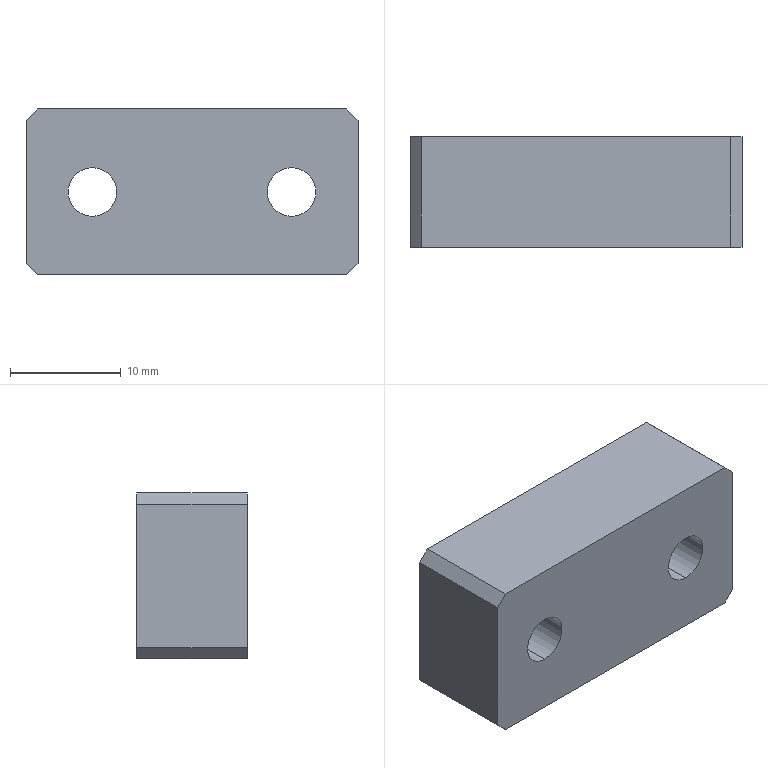Part | STEP file | PN_0004 | 1 solid | 14 faces | box 30 x 10 x 15 mm | volume 4176 mm3 | plane 10 | cylinder 4 | commonest cylinder face diameters 4.4 x4
STEP:
#1=CARTESIAN_POINT('',(0.,0.,0.));
#2=DIRECTION('',(0.,0.,1.));
#3=DIRECTION('',(1.,0.,0.));
#4=AXIS2_PLACEMENT_3D('',#1,#2,#3);
#5=CARTESIAN_POINT('',(9.,10.,-2.2));
#6=VERTEX_POINT('',#5);
#7=CARTESIAN_POINT('',(9.,0.,-2.2));
#8=VERTEX_POINT('',#7);
#9=CARTESIAN_POINT('',(9.,0.,-2.2));
#10=DIRECTION('',(0.,-1.,0.));
#11=VECTOR('',#10,1.);
#12=LINE('',#9,#11);
#13=CARTESIAN_POINT('',(9.,0.,0.));
#14=DIRECTION('',(0.,-1.,0.));
#15=DIRECTION('',(0.,0.,-1.));
#16=AXIS2_PLACEMENT_3D('',#13,#14,#15);
#17=CYLINDRICAL_SURFACE('',#16,2.2);
#18=CARTESIAN_POINT('',(6.283,0.));
#19=DIRECTION('',(0.,1.));
#20=VECTOR('',#19,1.);
#21=LINE('',#18,#20);
#22=(GEOMETRIC_REPRESENTATION_CONTEXT(2)PARAMETRIC_REPRESENTATION_CONTEXT()REPRESENTATION_CONTEXT('',''));
#23=DEFINITIONAL_REPRESENTATION('',(#21),#22);
#24=PCURVE('',#17,#23);
#25=CARTESIAN_POINT('',(9.,0.,0.));
#26=DIRECTION('',(0.,-1.,0.));
#27=DIRECTION('',(0.,0.,-1.));
#28=AXIS2_PLACEMENT_3D('',#25,#26,#27);
#29=CYLINDRICAL_SURFACE('',#28,2.2);
#30=CARTESIAN_POINT('',(0.,0.));
#31=DIRECTION('',(0.,1.));
#32=VECTOR('',#31,1.);
#33=LINE('',#30,#32);
#34=(GEOMETRIC_REPRESENTATION_CONTEXT(2)PARAMETRIC_REPRESENTATION_CONTEXT()REPRESENTATION_CONTEXT('',''));
#35=DEFINITIONAL_REPRESENTATION('',(#33),#34);
#36=PCURVE('',#29,#35);
#37=SURFACE_CURVE('',#12,(#24,#36),.PCURVE_S1.);
#38=EDGE_CURVE('',#6,#8,#37,.T.);
#39=ORIENTED_EDGE('',*,*,#38,.T.);
#40=CARTESIAN_POINT('',(9.,0.,2.2));
#41=VERTEX_POINT('',#40);
#42=CARTESIAN_POINT('',(9.,0.,0.));
#43=DIRECTION('',(0.,-1.,0.));
#44=DIRECTION('',(0.,0.,-1.));
#45=AXIS2_PLACEMENT_3D('',#42,#43,#44);
#46=CIRCLE('',#45,2.2);
#47=CARTESIAN_POINT('',(0.,0.));
#48=DIRECTION('',(1.,0.));
#49=VECTOR('',#48,1.);
#50=LINE('',#47,#49);
#51=(GEOMETRIC_REPRESENTATION_CONTEXT(2)PARAMETRIC_REPRESENTATION_CONTEXT()REPRESENTATION_CONTEXT('',''));
#52=DEFINITIONAL_REPRESENTATION('',(#50),#51);
#53=PCURVE('',#17,#52);
#54=CARTESIAN_POINT('',(0.,0.,0.));
#55=DIRECTION('',(0.,1.,0.));
#56=DIRECTION('',(0.,0.,1.));
#57=AXIS2_PLACEMENT_3D('',#54,#55,#56);
#58=PLANE('',#57);
#59=CARTESIAN_POINT('',(-2.2,9.));
#60=CARTESIAN_POINT('',(-2.2,12.811));
#61=CARTESIAN_POINT('',(1.1,10.905));
#62=CARTESIAN_POINT('',(4.4,9.));
#63=CARTESIAN_POINT('',(1.1,7.095));
#64=CARTESIAN_POINT('',(-2.2,5.189));
#65=CARTESIAN_POINT('',(-2.2,9.));
#66=(BOUNDED_CURVE()B_SPLINE_CURVE(2,(#59,#60,#61,#62,#63,#64,#65),.UNSPECIFIED.,.T.,.F.)B_SPLINE_CURVE_WITH_KNOTS((1,2,2,2,2,1),(-2.094,0.,2.094,4.189,6.283,8.378),.UNSPECIFIED.)CURVE()GEOMETRIC_REPRESENTATION_ITEM()RATIONAL_B_SPLINE_CURVE((1.,0.5,1.,0.5,1.,0.5,1.))REPRESENTATION_ITEM(''));
#67=(GEOMETRIC_REPRESENTATION_CONTEXT(2)PARAMETRIC_REPRESENTATION_CONTEXT()REPRESENTATION_CONTEXT('',''));
#68=DEFINITIONAL_REPRESENTATION('',(#66),#67);
#69=PCURVE('',#58,#68);
#70=SURFACE_CURVE('',#46,(#53,#69),.PCURVE_S1.);
#71=EDGE_CURVE('',#41,#8,#70,.T.);
#72=ORIENTED_EDGE('',*,*,#71,.F.);
#73=CARTESIAN_POINT('',(9.,10.,2.2));
#74=VERTEX_POINT('',#73);
#75=CARTESIAN_POINT('',(9.,0.,2.2));
#76=DIRECTION('',(0.,-1.,0.));
#77=VECTOR('',#76,1.);
#78=LINE('',#75,#77);
#79=CARTESIAN_POINT('',(3.142,0.));
#80=DIRECTION('',(0.,1.));
#81=VECTOR('',#80,1.);
#82=LINE('',#79,#81);
#83=(GEOMETRIC_REPRESENTATION_CONTEXT(2)PARAMETRIC_REPRESENTATION_CONTEXT()REPRESENTATION_CONTEXT('',''));
#84=DEFINITIONAL_REPRESENTATION('',(#82),#83);
#85=PCURVE('',#17,#84);
#86=CARTESIAN_POINT('',(3.142,0.));
#87=DIRECTION('',(0.,1.));
#88=VECTOR('',#87,1.);
#89=LINE('',#86,#88);
#90=(GEOMETRIC_REPRESENTATION_CONTEXT(2)PARAMETRIC_REPRESENTATION_CONTEXT()REPRESENTATION_CONTEXT('',''));
#91=DEFINITIONAL_REPRESENTATION('',(#89),#90);
#92=PCURVE('',#29,#91);
#93=SURFACE_CURVE('',#78,(#85,#92),.PCURVE_S1.);
#94=EDGE_CURVE('',#74,#41,#93,.T.);
#95=ORIENTED_EDGE('',*,*,#94,.F.);
#96=CARTESIAN_POINT('',(9.,10.,0.));
#97=DIRECTION('',(0.,-1.,0.));
#98=DIRECTION('',(0.,0.,-1.));
#99=AXIS2_PLACEMENT_3D('',#96,#97,#98);
#100=CIRCLE('',#99,2.2);
#101=CARTESIAN_POINT('',(0.,-10.));
#102=DIRECTION('',(1.,0.));
#103=VECTOR('',#102,1.);
#104=LINE('',#101,#103);
#105=(GEOMETRIC_REPRESENTATION_CONTEXT(2)PARAMETRIC_REPRESENTATION_CONTEXT()REPRESENTATION_CONTEXT('',''));
#106=DEFINITIONAL_REPRESENTATION('',(#104),#105);
#107=PCURVE('',#17,#106);
#108=CARTESIAN_POINT('',(0.,10.,0.));
#109=DIRECTION('',(0.,1.,0.));
#110=DIRECTION('',(0.,0.,1.));
#111=AXIS2_PLACEMENT_3D('',#108,#109,#110);
#112=PLANE('',#111);
#113=CARTESIAN_POINT('',(-2.2,9.));
#114=CARTESIAN_POINT('',(-2.2,12.811));
#115=CARTESIAN_POINT('',(1.1,10.905));
#116=CARTESIAN_POINT('',(4.4,9.));
#117=CARTESIAN_POINT('',(1.1,7.095));
#118=CARTESIAN_POINT('',(-2.2,5.189));
#119=CARTESIAN_POINT('',(-2.2,9.));
#120=(BOUNDED_CURVE()B_SPLINE_CURVE(2,(#113,#114,#115,#116,#117,#118,#119),.UNSPECIFIED.,.T.,.F.)B_SPLINE_CURVE_WITH_KNOTS((1,2,2,2,2,1),(-2.094,0.,2.094,4.189,6.283,8.378),.UNSPECIFIED.)CURVE()GEOMETRIC_REPRESENTATION_ITEM()RATIONAL_B_SPLINE_CURVE((1.,0.5,1.,0.5,1.,0.5,1.))REPRESENTATION_ITEM(''));
#121=(GEOMETRIC_REPRESENTATION_CONTEXT(2)PARAMETRIC_REPRESENTATION_CONTEXT()REPRESENTATION_CONTEXT('',''));
#122=DEFINITIONAL_REPRESENTATION('',(#120),#121);
#123=PCURVE('',#112,#122);
#124=SURFACE_CURVE('',#100,(#107,#123),.PCURVE_S1.);
#125=EDGE_CURVE('',#74,#6,#124,.T.);
#126=ORIENTED_EDGE('',*,*,#125,.T.);
#127=EDGE_LOOP('',(#39,#72,#95,#126));
#128=FACE_BOUND('',#127,.F.);
#129=ADVANCED_FACE('',(#128),#17,.F.);
#130=CARTESIAN_POINT('',(-9.,10.,-2.2));
#131=VERTEX_POINT('',#130);
#132=CARTESIAN_POINT('',(-9.,0.,-2.2));
#133=VERTEX_POINT('',#132);
#134=CARTESIAN_POINT('',(-9.,0.,-2.2));
#135=DIRECTION('',(0.,-1.,0.));
#136=VECTOR('',#135,1.);
#137=LINE('',#134,#136);
#138=CARTESIAN_POINT('',(-9.,0.,0.));
#139=DIRECTION('',(0.,-1.,0.));
#140=DIRECTION('',(0.,0.,-1.));
#141=AXIS2_PLACEMENT_3D('',#138,#139,#140);
#142=CYLINDRICAL_SURFACE('',#141,2.2);
#143=CARTESIAN_POINT('',(6.283,0.));
#144=DIRECTION('',(0.,1.));
#145=VECTOR('',#144,1.);
#146=LINE('',#143,#145);
#147=(GEOMETRIC_REPRESENTATION_CONTEXT(2)PARAMETRIC_REPRESENTATION_CONTEXT()REPRESENTATION_CONTEXT('',''));
#148=DEFINITIONAL_REPRESENTATION('',(#146),#147);
#149=PCURVE('',#142,#148);
#150=CARTESIAN_POINT('',(-9.,0.,0.));
#151=DIRECTION('',(0.,-1.,0.));
#152=DIRECTION('',(0.,0.,-1.));
#153=AXIS2_PLACEMENT_3D('',#150,#151,#152);
#154=CYLINDRICAL_SURFACE('',#153,2.2);
#155=CARTESIAN_POINT('',(0.,0.));
#156=DIRECTION('',(0.,1.));
#157=VECTOR('',#156,1.);
#158=LINE('',#155,#157);
#159=(GEOMETRIC_REPRESENTATION_CONTEXT(2)PARAMETRIC_REPRESENTATION_CONTEXT()REPRESENTATION_CONTEXT('',''));
#160=DEFINITIONAL_REPRESENTATION('',(#158),#159);
#161=PCURVE('',#154,#160);
#162=SURFACE_CURVE('',#137,(#149,#161),.PCURVE_S1.);
#163=EDGE_CURVE('',#131,#133,#162,.T.);
#164=ORIENTED_EDGE('',*,*,#163,.T.);
#165=CARTESIAN_POINT('',(-9.,0.,2.2));
#166=VERTEX_POINT('',#165);
#167=CARTESIAN_POINT('',(-9.,0.,0.));
#168=DIRECTION('',(0.,-1.,0.));
#169=DIRECTION('',(0.,0.,-1.));
#170=AXIS2_PLACEMENT_3D('',#167,#168,#169);
#171=CIRCLE('',#170,2.2);
#172=CARTESIAN_POINT('',(0.,0.));
#173=DIRECTION('',(1.,0.));
#174=VECTOR('',#173,1.);
#175=LINE('',#172,#174);
#176=(GEOMETRIC_REPRESENTATION_CONTEXT(2)PARAMETRIC_REPRESENTATION_CONTEXT()REPRESENTATION_CONTEXT('',''));
#177=DEFINITIONAL_REPRESENTATION('',(#175),#176);
#178=PCURVE('',#142,#177);
#179=CARTESIAN_POINT('',(-2.2,-9.));
#180=CARTESIAN_POINT('',(-2.2,-5.189));
#181=CARTESIAN_POINT('',(1.1,-7.095));
#182=CARTESIAN_POINT('',(4.4,-9.));
#183=CARTESIAN_POINT('',(1.1,-10.905));
#184=CARTESIAN_POINT('',(-2.2,-12.811));
#185=CARTESIAN_POINT('',(-2.2,-9.));
#186=(BOUNDED_CURVE()B_SPLINE_CURVE(2,(#179,#180,#181,#182,#183,#184,#185),.UNSPECIFIED.,.T.,.F.)B_SPLINE_CURVE_WITH_KNOTS((1,2,2,2,2,1),(-2.094,0.,2.094,4.189,6.283,8.378),.UNSPECIFIED.)CURVE()GEOMETRIC_REPRESENTATION_ITEM()RATIONAL_B_SPLINE_CURVE((1.,0.5,1.,0.5,1.,0.5,1.))REPRESENTATION_ITEM(''));
#187=(GEOMETRIC_REPRESENTATION_CONTEXT(2)PARAMETRIC_REPRESENTATION_CONTEXT()REPRESENTATION_CONTEXT('',''));
#188=DEFINITIONAL_REPRESENTATION('',(#186),#187);
#189=PCURVE('',#58,#188);
#190=SURFACE_CURVE('',#171,(#178,#189),.PCURVE_S1.);
#191=EDGE_CURVE('',#166,#133,#190,.T.);
#192=ORIENTED_EDGE('',*,*,#191,.F.);
#193=CARTESIAN_POINT('',(-9.,10.,2.2));
#194=VERTEX_POINT('',#193);
#195=CARTESIAN_POINT('',(-9.,0.,2.2));
#196=DIRECTION('',(0.,-1.,0.));
#197=VECTOR('',#196,1.);
#198=LINE('',#195,#197);
#199=CARTESIAN_POINT('',(3.142,0.));
#200=DIRECTION('',(0.,1.));
#201=VECTOR('',#200,1.);
#202=LINE('',#199,#201);
#203=(GEOMETRIC_REPRESENTATION_CONTEXT(2)PARAMETRIC_REPRESENTATION_CONTEXT()REPRESENTATION_CONTEXT('',''));
#204=DEFINITIONAL_REPRESENTATION('',(#202),#203);
#205=PCURVE('',#142,#204);
#206=CARTESIAN_POINT('',(3.142,0.));
#207=DIRECTION('',(0.,1.));
#208=VECTOR('',#207,1.);
#209=LINE('',#206,#208);
#210=(GEOMETRIC_REPRESENTATION_CONTEXT(2)PARAMETRIC_REPRESENTATION_CONTEXT()REPRESENTATION_CONTEXT('',''));
#211=DEFINITIONAL_REPRESENTATION('',(#209),#210);
#212=PCURVE('',#154,#211);
#213=SURFACE_CURVE('',#198,(#205,#212),.PCURVE_S1.);
#214=EDGE_CURVE('',#194,#166,#213,.T.);
#215=ORIENTED_EDGE('',*,*,#214,.F.);
#216=CARTESIAN_POINT('',(-9.,10.,0.));
#217=DIRECTION('',(0.,-1.,0.));
#218=DIRECTION('',(0.,0.,-1.));
#219=AXIS2_PLACEMENT_3D('',#216,#217,#218);
#220=CIRCLE('',#219,2.2);
#221=CARTESIAN_POINT('',(0.,-10.));
#222=DIRECTION('',(1.,0.));
#223=VECTOR('',#222,1.);
#224=LINE('',#221,#223);
#225=(GEOMETRIC_REPRESENTATION_CONTEXT(2)PARAMETRIC_REPRESENTATION_CONTEXT()REPRESENTATION_CONTEXT('',''));
#226=DEFINITIONAL_REPRESENTATION('',(#224),#225);
#227=PCURVE('',#142,#226);
#228=CARTESIAN_POINT('',(-2.2,-9.));
#229=CARTESIAN_POINT('',(-2.2,-5.189));
#230=CARTESIAN_POINT('',(1.1,-7.095));
#231=CARTESIAN_POINT('',(4.4,-9.));
#232=CARTESIAN_POINT('',(1.1,-10.905));
#233=CARTESIAN_POINT('',(-2.2,-12.811));
#234=CARTESIAN_POINT('',(-2.2,-9.));
#235=(BOUNDED_CURVE()B_SPLINE_CURVE(2,(#228,#229,#230,#231,#232,#233,#234),.UNSPECIFIED.,.T.,.F.)B_SPLINE_CURVE_WITH_KNOTS((1,2,2,2,2,1),(-2.094,0.,2.094,4.189,6.283,8.378),.UNSPECIFIED.)CURVE()GEOMETRIC_REPRESENTATION_ITEM()RATIONAL_B_SPLINE_CURVE((1.,0.5,1.,0.5,1.,0.5,1.))REPRESENTATION_ITEM(''));
#236=(GEOMETRIC_REPRESENTATION_CONTEXT(2)PARAMETRIC_REPRESENTATION_CONTEXT()REPRESENTATION_CONTEXT('',''));
#237=DEFINITIONAL_REPRESENTATION('',(#235),#236);
#238=PCURVE('',#112,#237);
#239=SURFACE_CURVE('',#220,(#227,#238),.PCURVE_S1.);
#240=EDGE_CURVE('',#194,#131,#239,.T.);
#241=ORIENTED_EDGE('',*,*,#240,.T.);
#242=EDGE_LOOP('',(#164,#192,#215,#241));
#243=FACE_BOUND('',#242,.F.);
#244=ADVANCED_FACE('',(#243),#142,.F.);
#245=CARTESIAN_POINT('',(15.,0.,6.5));
#246=VERTEX_POINT('',#245);
#247=CARTESIAN_POINT('',(15.,0.,-6.5));
#248=VERTEX_POINT('',#247);
#249=CARTESIAN_POINT('',(15.,0.,-7.5));
#250=DIRECTION('',(0.,0.,-1.));
#251=VECTOR('',#250,1.);
#252=LINE('',#249,#251);
#253=CARTESIAN_POINT('',(15.,10.,-7.5));
#254=DIRECTION('',(-1.,0.,0.));
#255=DIRECTION('',(0.,0.,1.));
#256=AXIS2_PLACEMENT_3D('',#253,#254,#255);
#257=PLANE('',#256);
#258=CARTESIAN_POINT('',(0.,-10.));
#259=DIRECTION('',(-1.,0.));
#260=VECTOR('',#259,1.);
#261=LINE('',#258,#260);
#262=(GEOMETRIC_REPRESENTATION_CONTEXT(2)PARAMETRIC_REPRESENTATION_CONTEXT()REPRESENTATION_CONTEXT('',''));
#263=DEFINITIONAL_REPRESENTATION('',(#261),#262);
#264=PCURVE('',#257,#263);
#265=CARTESIAN_POINT('',(-7.5,15.));
#266=DIRECTION('',(-1.,0.));
#267=VECTOR('',#266,1.);
#268=LINE('',#265,#267);
#269=(GEOMETRIC_REPRESENTATION_CONTEXT(2)PARAMETRIC_REPRESENTATION_CONTEXT()REPRESENTATION_CONTEXT('',''));
#270=DEFINITIONAL_REPRESENTATION('',(#268),#269);
#271=PCURVE('',#58,#270);
#272=SURFACE_CURVE('',#252,(#264,#271),.PCURVE_S1.);
#273=EDGE_CURVE('',#246,#248,#272,.T.);
#274=ORIENTED_EDGE('',*,*,#273,.T.);
#275=CARTESIAN_POINT('',(15.,10.,-6.5));
#276=VERTEX_POINT('',#275);
#277=CARTESIAN_POINT('',(15.,10.,-6.5));
#278=DIRECTION('',(0.,1.,0.));
#279=VECTOR('',#278,1.);
#280=LINE('',#277,#279);
#281=CARTESIAN_POINT('',(1.,0.));
#282=DIRECTION('',(0.,1.));
#283=VECTOR('',#282,1.);
#284=LINE('',#281,#283);
#285=(GEOMETRIC_REPRESENTATION_CONTEXT(2)PARAMETRIC_REPRESENTATION_CONTEXT()REPRESENTATION_CONTEXT('',''));
#286=DEFINITIONAL_REPRESENTATION('',(#284),#285);
#287=PCURVE('',#257,#286);
#288=CARTESIAN_POINT('',(14.,10.,-7.5));
#289=DIRECTION('',(-0.7071,0.,0.7071));
#290=DIRECTION('',(0.,-1.,0.));
#291=AXIS2_PLACEMENT_3D('',#288,#289,#290);
#292=PLANE('',#291);
#293=CARTESIAN_POINT('',(0.,1.414));
#294=DIRECTION('',(-1.,0.));
#295=VECTOR('',#294,1.);
#296=LINE('',#293,#295);
#297=(GEOMETRIC_REPRESENTATION_CONTEXT(2)PARAMETRIC_REPRESENTATION_CONTEXT()REPRESENTATION_CONTEXT('',''));
#298=DEFINITIONAL_REPRESENTATION('',(#296),#297);
#299=PCURVE('',#292,#298);
#300=SURFACE_CURVE('',#280,(#287,#299),.PCURVE_S1.);
#301=EDGE_CURVE('',#248,#276,#300,.T.);
#302=ORIENTED_EDGE('',*,*,#301,.T.);
#303=CARTESIAN_POINT('',(15.,10.,6.5));
#304=VERTEX_POINT('',#303);
#305=CARTESIAN_POINT('',(15.,10.,-7.5));
#306=DIRECTION('',(0.,0.,-1.));
#307=VECTOR('',#306,1.);
#308=LINE('',#305,#307);
#309=CARTESIAN_POINT('',(0.,0.));
#310=DIRECTION('',(-1.,0.));
#311=VECTOR('',#310,1.);
#312=LINE('',#309,#311);
#313=(GEOMETRIC_REPRESENTATION_CONTEXT(2)PARAMETRIC_REPRESENTATION_CONTEXT()REPRESENTATION_CONTEXT('',''));
#314=DEFINITIONAL_REPRESENTATION('',(#312),#313);
#315=PCURVE('',#257,#314);
#316=CARTESIAN_POINT('',(-7.5,15.));
#317=DIRECTION('',(-1.,0.));
#318=VECTOR('',#317,1.);
#319=LINE('',#316,#318);
#320=(GEOMETRIC_REPRESENTATION_CONTEXT(2)PARAMETRIC_REPRESENTATION_CONTEXT()REPRESENTATION_CONTEXT('',''));
#321=DEFINITIONAL_REPRESENTATION('',(#319),#320);
#322=PCURVE('',#112,#321);
#323=SURFACE_CURVE('',#308,(#315,#322),.PCURVE_S1.);
#324=EDGE_CURVE('',#304,#276,#323,.T.);
#325=ORIENTED_EDGE('',*,*,#324,.F.);
#326=CARTESIAN_POINT('',(15.,10.,6.5));
#327=DIRECTION('',(0.,-1.,0.));
#328=VECTOR('',#327,1.);
#329=LINE('',#326,#328);
#330=CARTESIAN_POINT('',(14.,0.));
#331=DIRECTION('',(0.,-1.));
#332=VECTOR('',#331,1.);
#333=LINE('',#330,#332);
#334=(GEOMETRIC_REPRESENTATION_CONTEXT(2)PARAMETRIC_REPRESENTATION_CONTEXT()REPRESENTATION_CONTEXT('',''));
#335=DEFINITIONAL_REPRESENTATION('',(#333),#334);
#336=PCURVE('',#257,#335);
#337=CARTESIAN_POINT('',(15.,10.,6.5));
#338=DIRECTION('',(-0.7071,0.,-0.7071));
#339=DIRECTION('',(0.,-1.,0.));
#340=AXIS2_PLACEMENT_3D('',#337,#338,#339);
#341=PLANE('',#340);
#342=CARTESIAN_POINT('',(0.,0.));
#343=DIRECTION('',(1.,0.));
#344=VECTOR('',#343,1.);
#345=LINE('',#342,#344);
#346=(GEOMETRIC_REPRESENTATION_CONTEXT(2)PARAMETRIC_REPRESENTATION_CONTEXT()REPRESENTATION_CONTEXT('',''));
#347=DEFINITIONAL_REPRESENTATION('',(#345),#346);
#348=PCURVE('',#341,#347);
#349=SURFACE_CURVE('',#329,(#336,#348),.PCURVE_S1.);
#350=EDGE_CURVE('',#304,#246,#349,.T.);
#351=ORIENTED_EDGE('',*,*,#350,.T.);
#352=EDGE_LOOP('',(#274,#302,#325,#351));
#353=FACE_BOUND('',#352,.T.);
#354=ADVANCED_FACE('',(#353),#257,.F.);
#355=CARTESIAN_POINT('',(14.,0.,-7.5));
#356=VERTEX_POINT('',#355);
#357=CARTESIAN_POINT('',(-14.,0.,-7.5));
#358=VERTEX_POINT('',#357);
#359=CARTESIAN_POINT('',(-15.,0.,-7.5));
#360=DIRECTION('',(-1.,0.,0.));
#361=VECTOR('',#360,1.);
#362=LINE('',#359,#361);
#363=CARTESIAN_POINT('',(-15.,10.,-7.5));
#364=DIRECTION('',(0.,0.,1.));
#365=DIRECTION('',(1.,0.,0.));
#366=AXIS2_PLACEMENT_3D('',#363,#364,#365);
#367=PLANE('',#366);
#368=CARTESIAN_POINT('',(0.,-10.));
#369=DIRECTION('',(-1.,0.));
#370=VECTOR('',#369,1.);
#371=LINE('',#368,#370);
#372=(GEOMETRIC_REPRESENTATION_CONTEXT(2)PARAMETRIC_REPRESENTATION_CONTEXT()REPRESENTATION_CONTEXT('',''));
#373=DEFINITIONAL_REPRESENTATION('',(#371),#372);
#374=PCURVE('',#367,#373);
#375=CARTESIAN_POINT('',(-7.5,-15.));
#376=DIRECTION('',(0.,-1.));
#377=VECTOR('',#376,1.);
#378=LINE('',#375,#377);
#379=(GEOMETRIC_REPRESENTATION_CONTEXT(2)PARAMETRIC_REPRESENTATION_CONTEXT()REPRESENTATION_CONTEXT('',''));
#380=DEFINITIONAL_REPRESENTATION('',(#378),#379);
#381=PCURVE('',#58,#380);
#382=SURFACE_CURVE('',#362,(#374,#381),.PCURVE_S1.);
#383=EDGE_CURVE('',#356,#358,#382,.T.);
#384=ORIENTED_EDGE('',*,*,#383,.T.);
#385=CARTESIAN_POINT('',(-14.,10.,-7.5));
#386=VERTEX_POINT('',#385);
#387=CARTESIAN_POINT('',(-14.,10.,-7.5));
#388=DIRECTION('',(0.,1.,0.));
#389=VECTOR('',#388,1.);
#390=LINE('',#387,#389);
#391=CARTESIAN_POINT('',(1.,0.));
#392=DIRECTION('',(0.,1.));
#393=VECTOR('',#392,1.);
#394=LINE('',#391,#393);
#395=(GEOMETRIC_REPRESENTATION_CONTEXT(2)PARAMETRIC_REPRESENTATION_CONTEXT()REPRESENTATION_CONTEXT('',''));
#396=DEFINITIONAL_REPRESENTATION('',(#394),#395);
#397=PCURVE('',#367,#396);
#398=CARTESIAN_POINT('',(-15.,10.,-6.5));
#399=DIRECTION('',(0.7071,0.,0.7071));
#400=DIRECTION('',(0.,-1.,0.));
#401=AXIS2_PLACEMENT_3D('',#398,#399,#400);
#402=PLANE('',#401);
#403=CARTESIAN_POINT('',(0.,1.414));
#404=DIRECTION('',(-1.,0.));
#405=VECTOR('',#404,1.);
#406=LINE('',#403,#405);
#407=(GEOMETRIC_REPRESENTATION_CONTEXT(2)PARAMETRIC_REPRESENTATION_CONTEXT()REPRESENTATION_CONTEXT('',''));
#408=DEFINITIONAL_REPRESENTATION('',(#406),#407);
#409=PCURVE('',#402,#408);
#410=SURFACE_CURVE('',#390,(#397,#409),.PCURVE_S1.);
#411=EDGE_CURVE('',#358,#386,#410,.T.);
#412=ORIENTED_EDGE('',*,*,#411,.T.);
#413=CARTESIAN_POINT('',(14.,10.,-7.5));
#414=VERTEX_POINT('',#413);
#415=CARTESIAN_POINT('',(-15.,10.,-7.5));
#416=DIRECTION('',(-1.,0.,0.));
#417=VECTOR('',#416,1.);
#418=LINE('',#415,#417);
#419=CARTESIAN_POINT('',(0.,0.));
#420=DIRECTION('',(-1.,0.));
#421=VECTOR('',#420,1.);
#422=LINE('',#419,#421);
#423=(GEOMETRIC_REPRESENTATION_CONTEXT(2)PARAMETRIC_REPRESENTATION_CONTEXT()REPRESENTATION_CONTEXT('',''));
#424=DEFINITIONAL_REPRESENTATION('',(#422),#423);
#425=PCURVE('',#367,#424);
#426=CARTESIAN_POINT('',(-7.5,-15.));
#427=DIRECTION('',(0.,-1.));
#428=VECTOR('',#427,1.);
#429=LINE('',#426,#428);
#430=(GEOMETRIC_REPRESENTATION_CONTEXT(2)PARAMETRIC_REPRESENTATION_CONTEXT()REPRESENTATION_CONTEXT('',''));
#431=DEFINITIONAL_REPRESENTATION('',(#429),#430);
#432=PCURVE('',#112,#431);
#433=SURFACE_CURVE('',#418,(#425,#432),.PCURVE_S1.);
#434=EDGE_CURVE('',#414,#386,#433,.T.);
#435=ORIENTED_EDGE('',*,*,#434,.F.);
#436=CARTESIAN_POINT('',(14.,10.,-7.5));
#437=DIRECTION('',(0.,-1.,0.));
#438=VECTOR('',#437,1.);
#439=LINE('',#436,#438);
#440=CARTESIAN_POINT('',(29.,0.));
#441=DIRECTION('',(0.,-1.));
#442=VECTOR('',#441,1.);
#443=LINE('',#440,#442);
#444=(GEOMETRIC_REPRESENTATION_CONTEXT(2)PARAMETRIC_REPRESENTATION_CONTEXT()REPRESENTATION_CONTEXT('',''));
#445=DEFINITIONAL_REPRESENTATION('',(#443),#444);
#446=PCURVE('',#367,#445);
#447=CARTESIAN_POINT('',(0.,0.));
#448=DIRECTION('',(1.,0.));
#449=VECTOR('',#448,1.);
#450=LINE('',#447,#449);
#451=(GEOMETRIC_REPRESENTATION_CONTEXT(2)PARAMETRIC_REPRESENTATION_CONTEXT()REPRESENTATION_CONTEXT('',''));
#452=DEFINITIONAL_REPRESENTATION('',(#450),#451);
#453=PCURVE('',#292,#452);
#454=SURFACE_CURVE('',#439,(#446,#453),.PCURVE_S1.);
#455=EDGE_CURVE('',#414,#356,#454,.T.);
#456=ORIENTED_EDGE('',*,*,#455,.T.);
#457=EDGE_LOOP('',(#384,#412,#435,#456));
#458=FACE_BOUND('',#457,.T.);
#459=ADVANCED_FACE('',(#458),#367,.F.);
#460=CARTESIAN_POINT('',(-15.,10.,-6.5));
#461=VERTEX_POINT('',#460);
#462=CARTESIAN_POINT('',(-15.,10.,6.5));
#463=VERTEX_POINT('',#462);
#464=CARTESIAN_POINT('',(-15.,10.,-7.5));
#465=DIRECTION('',(0.,0.,1.));
#466=VECTOR('',#465,1.);
#467=LINE('',#464,#466);
#468=CARTESIAN_POINT('',(-15.,10.,-7.5));
#469=DIRECTION('',(1.,0.,0.));
#470=DIRECTION('',(0.,0.,-1.));
#471=AXIS2_PLACEMENT_3D('',#468,#469,#470);
#472=PLANE('',#471);
#473=CARTESIAN_POINT('',(0.,0.));
#474=DIRECTION('',(-1.,0.));
#475=VECTOR('',#474,1.);
#476=LINE('',#473,#475);
#477=(GEOMETRIC_REPRESENTATION_CONTEXT(2)PARAMETRIC_REPRESENTATION_CONTEXT()REPRESENTATION_CONTEXT('',''));
#478=DEFINITIONAL_REPRESENTATION('',(#476),#477);
#479=PCURVE('',#472,#478);
#480=CARTESIAN_POINT('',(-7.5,-15.));
#481=DIRECTION('',(1.,0.));
#482=VECTOR('',#481,1.);
#483=LINE('',#480,#482);
#484=(GEOMETRIC_REPRESENTATION_CONTEXT(2)PARAMETRIC_REPRESENTATION_CONTEXT()REPRESENTATION_CONTEXT('',''));
#485=DEFINITIONAL_REPRESENTATION('',(#483),#484);
#486=PCURVE('',#112,#485);
#487=SURFACE_CURVE('',#467,(#479,#486),.PCURVE_S1.);
#488=EDGE_CURVE('',#461,#463,#487,.T.);
#489=ORIENTED_EDGE('',*,*,#488,.F.);
#490=CARTESIAN_POINT('',(-15.,0.,-6.5));
#491=VERTEX_POINT('',#490);
#492=CARTESIAN_POINT('',(-15.,10.,-6.5));
#493=DIRECTION('',(0.,-1.,0.));
#494=VECTOR('',#493,1.);
#495=LINE('',#492,#494);
#496=CARTESIAN_POINT('',(-1.,0.));
#497=DIRECTION('',(0.,-1.));
#498=VECTOR('',#497,1.);
#499=LINE('',#496,#498);
#500=(GEOMETRIC_REPRESENTATION_CONTEXT(2)PARAMETRIC_REPRESENTATION_CONTEXT()REPRESENTATION_CONTEXT('',''));
#501=DEFINITIONAL_REPRESENTATION('',(#499),#500);
#502=PCURVE('',#472,#501);
#503=CARTESIAN_POINT('',(0.,0.));
#504=DIRECTION('',(1.,0.));
#505=VECTOR('',#504,1.);
#506=LINE('',#503,#505);
#507=(GEOMETRIC_REPRESENTATION_CONTEXT(2)PARAMETRIC_REPRESENTATION_CONTEXT()REPRESENTATION_CONTEXT('',''));
#508=DEFINITIONAL_REPRESENTATION('',(#506),#507);
#509=PCURVE('',#402,#508);
#510=SURFACE_CURVE('',#495,(#502,#509),.PCURVE_S1.);
#511=EDGE_CURVE('',#461,#491,#510,.T.);
#512=ORIENTED_EDGE('',*,*,#511,.T.);
#513=CARTESIAN_POINT('',(-15.,0.,6.5));
#514=VERTEX_POINT('',#513);
#515=CARTESIAN_POINT('',(-15.,0.,-7.5));
#516=DIRECTION('',(0.,0.,1.));
#517=VECTOR('',#516,1.);
#518=LINE('',#515,#517);
#519=CARTESIAN_POINT('',(0.,-10.));
#520=DIRECTION('',(-1.,0.));
#521=VECTOR('',#520,1.);
#522=LINE('',#519,#521);
#523=(GEOMETRIC_REPRESENTATION_CONTEXT(2)PARAMETRIC_REPRESENTATION_CONTEXT()REPRESENTATION_CONTEXT('',''));
#524=DEFINITIONAL_REPRESENTATION('',(#522),#523);
#525=PCURVE('',#472,#524);
#526=CARTESIAN_POINT('',(-7.5,-15.));
#527=DIRECTION('',(1.,0.));
#528=VECTOR('',#527,1.);
#529=LINE('',#526,#528);
#530=(GEOMETRIC_REPRESENTATION_CONTEXT(2)PARAMETRIC_REPRESENTATION_CONTEXT()REPRESENTATION_CONTEXT('',''));
#531=DEFINITIONAL_REPRESENTATION('',(#529),#530);
#532=PCURVE('',#58,#531);
#533=SURFACE_CURVE('',#518,(#525,#532),.PCURVE_S1.);
#534=EDGE_CURVE('',#491,#514,#533,.T.);
#535=ORIENTED_EDGE('',*,*,#534,.T.);
#536=CARTESIAN_POINT('',(-15.,10.,6.5));
#537=DIRECTION('',(0.,1.,0.));
#538=VECTOR('',#537,1.);
#539=LINE('',#536,#538);
#540=CARTESIAN_POINT('',(-14.,0.));
#541=DIRECTION('',(0.,1.));
#542=VECTOR('',#541,1.);
#543=LINE('',#540,#542);
#544=(GEOMETRIC_REPRESENTATION_CONTEXT(2)PARAMETRIC_REPRESENTATION_CONTEXT()REPRESENTATION_CONTEXT('',''));
#545=DEFINITIONAL_REPRESENTATION('',(#543),#544);
#546=PCURVE('',#472,#545);
#547=CARTESIAN_POINT('',(-14.,10.,7.5));
#548=DIRECTION('',(0.7071,0.,-0.7071));
#549=DIRECTION('',(0.,-1.,0.));
#550=AXIS2_PLACEMENT_3D('',#547,#548,#549);
#551=PLANE('',#550);
#552=CARTESIAN_POINT('',(0.,1.414));
#553=DIRECTION('',(-1.,0.));
#554=VECTOR('',#553,1.);
#555=LINE('',#552,#554);
#556=(GEOMETRIC_REPRESENTATION_CONTEXT(2)PARAMETRIC_REPRESENTATION_CONTEXT()REPRESENTATION_CONTEXT('',''));
#557=DEFINITIONAL_REPRESENTATION('',(#555),#556);
#558=PCURVE('',#551,#557);
#559=SURFACE_CURVE('',#539,(#546,#558),.PCURVE_S1.);
#560=EDGE_CURVE('',#514,#463,#559,.T.);
#561=ORIENTED_EDGE('',*,*,#560,.T.);
#562=EDGE_LOOP('',(#489,#512,#535,#561));
#563=FACE_BOUND('',#562,.T.);
#564=ADVANCED_FACE('',(#563),#472,.F.);
#565=CARTESIAN_POINT('',(-14.,10.,7.5));
#566=VERTEX_POINT('',#565);
#567=CARTESIAN_POINT('',(14.,10.,7.5));
#568=VERTEX_POINT('',#567);
#569=CARTESIAN_POINT('',(-15.,10.,7.5));
#570=DIRECTION('',(1.,0.,0.));
#571=VECTOR('',#570,1.);
#572=LINE('',#569,#571);
#573=CARTESIAN_POINT('',(-15.,10.,7.5));
#574=DIRECTION('',(0.,0.,-1.));
#575=DIRECTION('',(-1.,0.,0.));
#576=AXIS2_PLACEMENT_3D('',#573,#574,#575);
#577=PLANE('',#576);
#578=CARTESIAN_POINT('',(0.,0.));
#579=DIRECTION('',(-1.,0.));
#580=VECTOR('',#579,1.);
#581=LINE('',#578,#580);
#582=(GEOMETRIC_REPRESENTATION_CONTEXT(2)PARAMETRIC_REPRESENTATION_CONTEXT()REPRESENTATION_CONTEXT('',''));
#583=DEFINITIONAL_REPRESENTATION('',(#581),#582);
#584=PCURVE('',#577,#583);
#585=CARTESIAN_POINT('',(7.5,-15.));
#586=DIRECTION('',(0.,1.));
#587=VECTOR('',#586,1.);
#588=LINE('',#585,#587);
#589=(GEOMETRIC_REPRESENTATION_CONTEXT(2)PARAMETRIC_REPRESENTATION_CONTEXT()REPRESENTATION_CONTEXT('',''));
#590=DEFINITIONAL_REPRESENTATION('',(#588),#589);
#591=PCURVE('',#112,#590);
#592=SURFACE_CURVE('',#572,(#584,#591),.PCURVE_S1.);
#593=EDGE_CURVE('',#566,#568,#592,.T.);
#594=ORIENTED_EDGE('',*,*,#593,.F.);
#595=CARTESIAN_POINT('',(-14.,0.,7.5));
#596=VERTEX_POINT('',#595);
#597=CARTESIAN_POINT('',(-14.,10.,7.5));
#598=DIRECTION('',(0.,-1.,0.));
#599=VECTOR('',#598,1.);
#600=LINE('',#597,#599);
#601=CARTESIAN_POINT('',(-1.,0.));
#602=DIRECTION('',(0.,-1.));
#603=VECTOR('',#602,1.);
#604=LINE('',#601,#603);
#605=(GEOMETRIC_REPRESENTATION_CONTEXT(2)PARAMETRIC_REPRESENTATION_CONTEXT()REPRESENTATION_CONTEXT('',''));
#606=DEFINITIONAL_REPRESENTATION('',(#604),#605);
#607=PCURVE('',#577,#606);
#608=CARTESIAN_POINT('',(0.,0.));
#609=DIRECTION('',(1.,0.));
#610=VECTOR('',#609,1.);
#611=LINE('',#608,#610);
#612=(GEOMETRIC_REPRESENTATION_CONTEXT(2)PARAMETRIC_REPRESENTATION_CONTEXT()REPRESENTATION_CONTEXT('',''));
#613=DEFINITIONAL_REPRESENTATION('',(#611),#612);
#614=PCURVE('',#551,#613);
#615=SURFACE_CURVE('',#600,(#607,#614),.PCURVE_S1.);
#616=EDGE_CURVE('',#566,#596,#615,.T.);
#617=ORIENTED_EDGE('',*,*,#616,.T.);
#618=CARTESIAN_POINT('',(14.,0.,7.5));
#619=VERTEX_POINT('',#618);
#620=CARTESIAN_POINT('',(-15.,0.,7.5));
#621=DIRECTION('',(1.,0.,0.));
#622=VECTOR('',#621,1.);
#623=LINE('',#620,#622);
#624=CARTESIAN_POINT('',(0.,-10.));
#625=DIRECTION('',(-1.,0.));
#626=VECTOR('',#625,1.);
#627=LINE('',#624,#626);
#628=(GEOMETRIC_REPRESENTATION_CONTEXT(2)PARAMETRIC_REPRESENTATION_CONTEXT()REPRESENTATION_CONTEXT('',''));
#629=DEFINITIONAL_REPRESENTATION('',(#627),#628);
#630=PCURVE('',#577,#629);
#631=CARTESIAN_POINT('',(7.5,-15.));
#632=DIRECTION('',(0.,1.));
#633=VECTOR('',#632,1.);
#634=LINE('',#631,#633);
#635=(GEOMETRIC_REPRESENTATION_CONTEXT(2)PARAMETRIC_REPRESENTATION_CONTEXT()REPRESENTATION_CONTEXT('',''));
#636=DEFINITIONAL_REPRESENTATION('',(#634),#635);
#637=PCURVE('',#58,#636);
#638=SURFACE_CURVE('',#623,(#630,#637),.PCURVE_S1.);
#639=EDGE_CURVE('',#596,#619,#638,.T.);
#640=ORIENTED_EDGE('',*,*,#639,.T.);
#641=CARTESIAN_POINT('',(14.,10.,7.5));
#642=DIRECTION('',(0.,1.,0.));
#643=VECTOR('',#642,1.);
#644=LINE('',#641,#643);
#645=CARTESIAN_POINT('',(-29.,0.));
#646=DIRECTION('',(0.,1.));
#647=VECTOR('',#646,1.);
#648=LINE('',#645,#647);
#649=(GEOMETRIC_REPRESENTATION_CONTEXT(2)PARAMETRIC_REPRESENTATION_CONTEXT()REPRESENTATION_CONTEXT('',''));
#650=DEFINITIONAL_REPRESENTATION('',(#648),#649);
#651=PCURVE('',#577,#650);
#652=CARTESIAN_POINT('',(0.,1.414));
#653=DIRECTION('',(-1.,0.));
#654=VECTOR('',#653,1.);
#655=LINE('',#652,#654);
#656=(GEOMETRIC_REPRESENTATION_CONTEXT(2)PARAMETRIC_REPRESENTATION_CONTEXT()REPRESENTATION_CONTEXT('',''));
#657=DEFINITIONAL_REPRESENTATION('',(#655),#656);
#658=PCURVE('',#341,#657);
#659=SURFACE_CURVE('',#644,(#651,#658),.PCURVE_S1.);
#660=EDGE_CURVE('',#619,#568,#659,.T.);
#661=ORIENTED_EDGE('',*,*,#660,.T.);
#662=EDGE_LOOP('',(#594,#617,#640,#661));
#663=FACE_BOUND('',#662,.T.);
#664=ADVANCED_FACE('',(#663),#577,.F.);
#665=CARTESIAN_POINT('',(9.,10.,0.));
#666=DIRECTION('',(0.,-1.,0.));
#667=DIRECTION('',(0.,0.,-1.));
#668=AXIS2_PLACEMENT_3D('',#665,#666,#667);
#669=CIRCLE('',#668,2.2);
#670=CARTESIAN_POINT('',(-2.2,9.));
#671=CARTESIAN_POINT('',(-2.2,12.811));
#672=CARTESIAN_POINT('',(1.1,10.905));
#673=CARTESIAN_POINT('',(4.4,9.));
#674=CARTESIAN_POINT('',(1.1,7.095));
#675=CARTESIAN_POINT('',(-2.2,5.189));
#676=CARTESIAN_POINT('',(-2.2,9.));
#677=(BOUNDED_CURVE()B_SPLINE_CURVE(2,(#670,#671,#672,#673,#674,#675,#676),.UNSPECIFIED.,.T.,.F.)B_SPLINE_CURVE_WITH_KNOTS((1,2,2,2,2,1),(-2.094,0.,2.094,4.189,6.283,8.378),.UNSPECIFIED.)CURVE()GEOMETRIC_REPRESENTATION_ITEM()RATIONAL_B_SPLINE_CURVE((1.,0.5,1.,0.5,1.,0.5,1.))REPRESENTATION_ITEM(''));
#678=(GEOMETRIC_REPRESENTATION_CONTEXT(2)PARAMETRIC_REPRESENTATION_CONTEXT()REPRESENTATION_CONTEXT('',''));
#679=DEFINITIONAL_REPRESENTATION('',(#677),#678);
#680=PCURVE('',#112,#679);
#681=CARTESIAN_POINT('',(0.,-10.));
#682=DIRECTION('',(1.,0.));
#683=VECTOR('',#682,1.);
#684=LINE('',#681,#683);
#685=(GEOMETRIC_REPRESENTATION_CONTEXT(2)PARAMETRIC_REPRESENTATION_CONTEXT()REPRESENTATION_CONTEXT('',''));
#686=DEFINITIONAL_REPRESENTATION('',(#684),#685);
#687=PCURVE('',#29,#686);
#688=SURFACE_CURVE('',#669,(#680,#687),.PCURVE_S1.);
#689=EDGE_CURVE('',#6,#74,#688,.T.);
#690=ORIENTED_EDGE('',*,*,#689,.T.);
#691=ORIENTED_EDGE('',*,*,#125,.T.);
#692=EDGE_LOOP('',(#690,#691));
#693=FACE_BOUND('',#692,.T.);
#694=CARTESIAN_POINT('',(-9.,10.,0.));
#695=DIRECTION('',(0.,-1.,0.));
#696=DIRECTION('',(0.,0.,-1.));
#697=AXIS2_PLACEMENT_3D('',#694,#695,#696);
#698=CIRCLE('',#697,2.2);
#699=CARTESIAN_POINT('',(-2.2,-9.));
#700=CARTESIAN_POINT('',(-2.2,-5.189));
#701=CARTESIAN_POINT('',(1.1,-7.095));
#702=CARTESIAN_POINT('',(4.4,-9.));
#703=CARTESIAN_POINT('',(1.1,-10.905));
#704=CARTESIAN_POINT('',(-2.2,-12.811));
#705=CARTESIAN_POINT('',(-2.2,-9.));
#706=(BOUNDED_CURVE()B_SPLINE_CURVE(2,(#699,#700,#701,#702,#703,#704,#705),.UNSPECIFIED.,.T.,.F.)B_SPLINE_CURVE_WITH_KNOTS((1,2,2,2,2,1),(-2.094,0.,2.094,4.189,6.283,8.378),.UNSPECIFIED.)CURVE()GEOMETRIC_REPRESENTATION_ITEM()RATIONAL_B_SPLINE_CURVE((1.,0.5,1.,0.5,1.,0.5,1.))REPRESENTATION_ITEM(''));
#707=(GEOMETRIC_REPRESENTATION_CONTEXT(2)PARAMETRIC_REPRESENTATION_CONTEXT()REPRESENTATION_CONTEXT('',''));
#708=DEFINITIONAL_REPRESENTATION('',(#706),#707);
#709=PCURVE('',#112,#708);
#710=CARTESIAN_POINT('',(0.,-10.));
#711=DIRECTION('',(1.,0.));
#712=VECTOR('',#711,1.);
#713=LINE('',#710,#712);
#714=(GEOMETRIC_REPRESENTATION_CONTEXT(2)PARAMETRIC_REPRESENTATION_CONTEXT()REPRESENTATION_CONTEXT('',''));
#715=DEFINITIONAL_REPRESENTATION('',(#713),#714);
#716=PCURVE('',#154,#715);
#717=SURFACE_CURVE('',#698,(#709,#716),.PCURVE_S1.);
#718=EDGE_CURVE('',#131,#194,#717,.T.);
#719=ORIENTED_EDGE('',*,*,#718,.T.);
#720=ORIENTED_EDGE('',*,*,#240,.T.);
#721=EDGE_LOOP('',(#719,#720));
#722=FACE_BOUND('',#721,.T.);
#723=ORIENTED_EDGE('',*,*,#434,.T.);
#724=CARTESIAN_POINT('',(-10.75,10.,-10.75));
#725=DIRECTION('',(-0.7071,0.,0.7071));
#726=VECTOR('',#725,1.);
#727=LINE('',#724,#726);
#728=CARTESIAN_POINT('',(-10.75,-10.75));
#729=DIRECTION('',(0.7071,-0.7071));
#730=VECTOR('',#729,1.);
#731=LINE('',#728,#730);
#732=(GEOMETRIC_REPRESENTATION_CONTEXT(2)PARAMETRIC_REPRESENTATION_CONTEXT()REPRESENTATION_CONTEXT('',''));
#733=DEFINITIONAL_REPRESENTATION('',(#731),#732);
#734=PCURVE('',#112,#733);
#735=CARTESIAN_POINT('',(0.,6.01));
#736=DIRECTION('',(0.,-1.));
#737=VECTOR('',#736,1.);
#738=LINE('',#735,#737);
#739=(GEOMETRIC_REPRESENTATION_CONTEXT(2)PARAMETRIC_REPRESENTATION_CONTEXT()REPRESENTATION_CONTEXT('',''));
#740=DEFINITIONAL_REPRESENTATION('',(#738),#739);
#741=PCURVE('',#402,#740);
#742=SURFACE_CURVE('',#727,(#734,#741),.PCURVE_S1.);
#743=EDGE_CURVE('',#386,#461,#742,.T.);
#744=ORIENTED_EDGE('',*,*,#743,.T.);
#745=ORIENTED_EDGE('',*,*,#488,.T.);
#746=CARTESIAN_POINT('',(-10.75,10.,10.75));
#747=DIRECTION('',(0.7071,0.,0.7071));
#748=VECTOR('',#747,1.);
#749=LINE('',#746,#748);
#750=CARTESIAN_POINT('',(10.75,-10.75));
#751=DIRECTION('',(0.7071,0.7071));
#752=VECTOR('',#751,1.);
#753=LINE('',#750,#752);
#754=(GEOMETRIC_REPRESENTATION_CONTEXT(2)PARAMETRIC_REPRESENTATION_CONTEXT()REPRESENTATION_CONTEXT('',''));
#755=DEFINITIONAL_REPRESENTATION('',(#753),#754);
#756=PCURVE('',#112,#755);
#757=CARTESIAN_POINT('',(0.,-4.596));
#758=DIRECTION('',(0.,-1.));
#759=VECTOR('',#758,1.);
#760=LINE('',#757,#759);
#761=(GEOMETRIC_REPRESENTATION_CONTEXT(2)PARAMETRIC_REPRESENTATION_CONTEXT()REPRESENTATION_CONTEXT('',''));
#762=DEFINITIONAL_REPRESENTATION('',(#760),#761);
#763=PCURVE('',#551,#762);
#764=SURFACE_CURVE('',#749,(#756,#763),.PCURVE_S1.);
#765=EDGE_CURVE('',#463,#566,#764,.T.);
#766=ORIENTED_EDGE('',*,*,#765,.T.);
#767=ORIENTED_EDGE('',*,*,#593,.T.);
#768=CARTESIAN_POINT('',(10.75,10.,10.75));
#769=DIRECTION('',(0.7071,0.,-0.7071));
#770=VECTOR('',#769,1.);
#771=LINE('',#768,#770);
#772=CARTESIAN_POINT('',(10.75,10.75));
#773=DIRECTION('',(-0.7071,0.7071));
#774=VECTOR('',#773,1.);
#775=LINE('',#772,#774);
#776=(GEOMETRIC_REPRESENTATION_CONTEXT(2)PARAMETRIC_REPRESENTATION_CONTEXT()REPRESENTATION_CONTEXT('',''));
#777=DEFINITIONAL_REPRESENTATION('',(#775),#776);
#778=PCURVE('',#112,#777);
#779=CARTESIAN_POINT('',(0.,6.01));
#780=DIRECTION('',(0.,-1.));
#781=VECTOR('',#780,1.);
#782=LINE('',#779,#781);
#783=(GEOMETRIC_REPRESENTATION_CONTEXT(2)PARAMETRIC_REPRESENTATION_CONTEXT()REPRESENTATION_CONTEXT('',''));
#784=DEFINITIONAL_REPRESENTATION('',(#782),#783);
#785=PCURVE('',#341,#784);
#786=SURFACE_CURVE('',#771,(#778,#785),.PCURVE_S1.);
#787=EDGE_CURVE('',#568,#304,#786,.T.);
#788=ORIENTED_EDGE('',*,*,#787,.T.);
#789=ORIENTED_EDGE('',*,*,#324,.T.);
#790=CARTESIAN_POINT('',(10.75,10.,-10.75));
#791=DIRECTION('',(-0.7071,0.,-0.7071));
#792=VECTOR('',#791,1.);
#793=LINE('',#790,#792);
#794=CARTESIAN_POINT('',(-10.75,10.75));
#795=DIRECTION('',(-0.7071,-0.7071));
#796=VECTOR('',#795,1.);
#797=LINE('',#794,#796);
#798=(GEOMETRIC_REPRESENTATION_CONTEXT(2)PARAMETRIC_REPRESENTATION_CONTEXT()REPRESENTATION_CONTEXT('',''));
#799=DEFINITIONAL_REPRESENTATION('',(#797),#798);
#800=PCURVE('',#112,#799);
#801=CARTESIAN_POINT('',(0.,-4.596));
#802=DIRECTION('',(0.,-1.));
#803=VECTOR('',#802,1.);
#804=LINE('',#801,#803);
#805=(GEOMETRIC_REPRESENTATION_CONTEXT(2)PARAMETRIC_REPRESENTATION_CONTEXT()REPRESENTATION_CONTEXT('',''));
#806=DEFINITIONAL_REPRESENTATION('',(#804),#805);
#807=PCURVE('',#292,#806);
#808=SURFACE_CURVE('',#793,(#800,#807),.PCURVE_S1.);
#809=EDGE_CURVE('',#276,#414,#808,.T.);
#810=ORIENTED_EDGE('',*,*,#809,.T.);
#811=EDGE_LOOP('',(#723,#744,#745,#766,#767,#788,#789,#810));
#812=FACE_BOUND('',#811,.T.);
#813=ADVANCED_FACE('',(#693,#722,#812),#112,.T.);
#814=CARTESIAN_POINT('',(9.,0.,0.));
#815=DIRECTION('',(0.,-1.,0.));
#816=DIRECTION('',(0.,0.,-1.));
#817=AXIS2_PLACEMENT_3D('',#814,#815,#816);
#818=CIRCLE('',#817,2.2);
#819=CARTESIAN_POINT('',(-2.2,9.));
#820=CARTESIAN_POINT('',(-2.2,12.811));
#821=CARTESIAN_POINT('',(1.1,10.905));
#822=CARTESIAN_POINT('',(4.4,9.));
#823=CARTESIAN_POINT('',(1.1,7.095));
#824=CARTESIAN_POINT('',(-2.2,5.189));
#825=CARTESIAN_POINT('',(-2.2,9.));
#826=(BOUNDED_CURVE()B_SPLINE_CURVE(2,(#819,#820,#821,#822,#823,#824,#825),.UNSPECIFIED.,.T.,.F.)B_SPLINE_CURVE_WITH_KNOTS((1,2,2,2,2,1),(-2.094,0.,2.094,4.189,6.283,8.378),.UNSPECIFIED.)CURVE()GEOMETRIC_REPRESENTATION_ITEM()RATIONAL_B_SPLINE_CURVE((1.,0.5,1.,0.5,1.,0.5,1.))REPRESENTATION_ITEM(''));
#827=(GEOMETRIC_REPRESENTATION_CONTEXT(2)PARAMETRIC_REPRESENTATION_CONTEXT()REPRESENTATION_CONTEXT('',''));
#828=DEFINITIONAL_REPRESENTATION('',(#826),#827);
#829=PCURVE('',#58,#828);
#830=CARTESIAN_POINT('',(0.,0.));
#831=DIRECTION('',(1.,0.));
#832=VECTOR('',#831,1.);
#833=LINE('',#830,#832);
#834=(GEOMETRIC_REPRESENTATION_CONTEXT(2)PARAMETRIC_REPRESENTATION_CONTEXT()REPRESENTATION_CONTEXT('',''));
#835=DEFINITIONAL_REPRESENTATION('',(#833),#834);
#836=PCURVE('',#29,#835);
#837=SURFACE_CURVE('',#818,(#829,#836),.PCURVE_S1.);
#838=EDGE_CURVE('',#8,#41,#837,.T.);
#839=ORIENTED_EDGE('',*,*,#838,.F.);
#840=ORIENTED_EDGE('',*,*,#71,.F.);
#841=EDGE_LOOP('',(#839,#840));
#842=FACE_BOUND('',#841,.T.);
#843=CARTESIAN_POINT('',(-9.,0.,0.));
#844=DIRECTION('',(0.,-1.,0.));
#845=DIRECTION('',(0.,0.,-1.));
#846=AXIS2_PLACEMENT_3D('',#843,#844,#845);
#847=CIRCLE('',#846,2.2);
#848=CARTESIAN_POINT('',(-2.2,-9.));
#849=CARTESIAN_POINT('',(-2.2,-5.189));
#850=CARTESIAN_POINT('',(1.1,-7.095));
#851=CARTESIAN_POINT('',(4.4,-9.));
#852=CARTESIAN_POINT('',(1.1,-10.905));
#853=CARTESIAN_POINT('',(-2.2,-12.811));
#854=CARTESIAN_POINT('',(-2.2,-9.));
#855=(BOUNDED_CURVE()B_SPLINE_CURVE(2,(#848,#849,#850,#851,#852,#853,#854),.UNSPECIFIED.,.T.,.F.)B_SPLINE_CURVE_WITH_KNOTS((1,2,2,2,2,1),(-2.094,0.,2.094,4.189,6.283,8.378),.UNSPECIFIED.)CURVE()GEOMETRIC_REPRESENTATION_ITEM()RATIONAL_B_SPLINE_CURVE((1.,0.5,1.,0.5,1.,0.5,1.))REPRESENTATION_ITEM(''));
#856=(GEOMETRIC_REPRESENTATION_CONTEXT(2)PARAMETRIC_REPRESENTATION_CONTEXT()REPRESENTATION_CONTEXT('',''));
#857=DEFINITIONAL_REPRESENTATION('',(#855),#856);
#858=PCURVE('',#58,#857);
#859=CARTESIAN_POINT('',(0.,0.));
#860=DIRECTION('',(1.,0.));
#861=VECTOR('',#860,1.);
#862=LINE('',#859,#861);
#863=(GEOMETRIC_REPRESENTATION_CONTEXT(2)PARAMETRIC_REPRESENTATION_CONTEXT()REPRESENTATION_CONTEXT('',''));
#864=DEFINITIONAL_REPRESENTATION('',(#862),#863);
#865=PCURVE('',#154,#864);
#866=SURFACE_CURVE('',#847,(#858,#865),.PCURVE_S1.);
#867=EDGE_CURVE('',#133,#166,#866,.T.);
#868=ORIENTED_EDGE('',*,*,#867,.F.);
#869=ORIENTED_EDGE('',*,*,#191,.F.);
#870=EDGE_LOOP('',(#868,#869));
#871=FACE_BOUND('',#870,.T.);
#872=ORIENTED_EDGE('',*,*,#534,.F.);
#873=CARTESIAN_POINT('',(-15.,0.,-6.5));
#874=DIRECTION('',(0.7071,0.,-0.7071));
#875=VECTOR('',#874,1.);
#876=LINE('',#873,#875);
#877=CARTESIAN_POINT('',(-6.5,-15.));
#878=DIRECTION('',(-0.7071,0.7071));
#879=VECTOR('',#878,1.);
#880=LINE('',#877,#879);
#881=(GEOMETRIC_REPRESENTATION_CONTEXT(2)PARAMETRIC_REPRESENTATION_CONTEXT()REPRESENTATION_CONTEXT('',''));
#882=DEFINITIONAL_REPRESENTATION('',(#880),#881);
#883=PCURVE('',#58,#882);
#884=CARTESIAN_POINT('',(10.,0.));
#885=DIRECTION('',(0.,1.));
#886=VECTOR('',#885,1.);
#887=LINE('',#884,#886);
#888=(GEOMETRIC_REPRESENTATION_CONTEXT(2)PARAMETRIC_REPRESENTATION_CONTEXT()REPRESENTATION_CONTEXT('',''));
#889=DEFINITIONAL_REPRESENTATION('',(#887),#888);
#890=PCURVE('',#402,#889);
#891=SURFACE_CURVE('',#876,(#883,#890),.PCURVE_S1.);
#892=EDGE_CURVE('',#491,#358,#891,.T.);
#893=ORIENTED_EDGE('',*,*,#892,.T.);
#894=ORIENTED_EDGE('',*,*,#383,.F.);
#895=CARTESIAN_POINT('',(14.,0.,-7.5));
#896=DIRECTION('',(0.7071,0.,0.7071));
#897=VECTOR('',#896,1.);
#898=LINE('',#895,#897);
#899=CARTESIAN_POINT('',(-7.5,14.));
#900=DIRECTION('',(0.7071,0.7071));
#901=VECTOR('',#900,1.);
#902=LINE('',#899,#901);
#903=(GEOMETRIC_REPRESENTATION_CONTEXT(2)PARAMETRIC_REPRESENTATION_CONTEXT()REPRESENTATION_CONTEXT('',''));
#904=DEFINITIONAL_REPRESENTATION('',(#902),#903);
#905=PCURVE('',#58,#904);
#906=CARTESIAN_POINT('',(10.,0.));
#907=DIRECTION('',(0.,1.));
#908=VECTOR('',#907,1.);
#909=LINE('',#906,#908);
#910=(GEOMETRIC_REPRESENTATION_CONTEXT(2)PARAMETRIC_REPRESENTATION_CONTEXT()REPRESENTATION_CONTEXT('',''));
#911=DEFINITIONAL_REPRESENTATION('',(#909),#910);
#912=PCURVE('',#292,#911);
#913=SURFACE_CURVE('',#898,(#905,#912),.PCURVE_S1.);
#914=EDGE_CURVE('',#356,#248,#913,.T.);
#915=ORIENTED_EDGE('',*,*,#914,.T.);
#916=ORIENTED_EDGE('',*,*,#273,.F.);
#917=CARTESIAN_POINT('',(15.,0.,6.5));
#918=DIRECTION('',(-0.7071,0.,0.7071));
#919=VECTOR('',#918,1.);
#920=LINE('',#917,#919);
#921=CARTESIAN_POINT('',(6.5,15.));
#922=DIRECTION('',(0.7071,-0.7071));
#923=VECTOR('',#922,1.);
#924=LINE('',#921,#923);
#925=(GEOMETRIC_REPRESENTATION_CONTEXT(2)PARAMETRIC_REPRESENTATION_CONTEXT()REPRESENTATION_CONTEXT('',''));
#926=DEFINITIONAL_REPRESENTATION('',(#924),#925);
#927=PCURVE('',#58,#926);
#928=CARTESIAN_POINT('',(10.,0.));
#929=DIRECTION('',(0.,1.));
#930=VECTOR('',#929,1.);
#931=LINE('',#928,#930);
#932=(GEOMETRIC_REPRESENTATION_CONTEXT(2)PARAMETRIC_REPRESENTATION_CONTEXT()REPRESENTATION_CONTEXT('',''));
#933=DEFINITIONAL_REPRESENTATION('',(#931),#932);
#934=PCURVE('',#341,#933);
#935=SURFACE_CURVE('',#920,(#927,#934),.PCURVE_S1.);
#936=EDGE_CURVE('',#246,#619,#935,.T.);
#937=ORIENTED_EDGE('',*,*,#936,.T.);
#938=ORIENTED_EDGE('',*,*,#639,.F.);
#939=CARTESIAN_POINT('',(-14.,0.,7.5));
#940=DIRECTION('',(-0.7071,0.,-0.7071));
#941=VECTOR('',#940,1.);
#942=LINE('',#939,#941);
#943=CARTESIAN_POINT('',(7.5,-14.));
#944=DIRECTION('',(-0.7071,-0.7071));
#945=VECTOR('',#944,1.);
#946=LINE('',#943,#945);
#947=(GEOMETRIC_REPRESENTATION_CONTEXT(2)PARAMETRIC_REPRESENTATION_CONTEXT()REPRESENTATION_CONTEXT('',''));
#948=DEFINITIONAL_REPRESENTATION('',(#946),#947);
#949=PCURVE('',#58,#948);
#950=CARTESIAN_POINT('',(10.,0.));
#951=DIRECTION('',(0.,1.));
#952=VECTOR('',#951,1.);
#953=LINE('',#950,#952);
#954=(GEOMETRIC_REPRESENTATION_CONTEXT(2)PARAMETRIC_REPRESENTATION_CONTEXT()REPRESENTATION_CONTEXT('',''));
#955=DEFINITIONAL_REPRESENTATION('',(#953),#954);
#956=PCURVE('',#551,#955);
#957=SURFACE_CURVE('',#942,(#949,#956),.PCURVE_S1.);
#958=EDGE_CURVE('',#596,#514,#957,.T.);
#959=ORIENTED_EDGE('',*,*,#958,.T.);
#960=EDGE_LOOP('',(#872,#893,#894,#915,#916,#937,#938,#959));
#961=FACE_BOUND('',#960,.T.);
#962=ADVANCED_FACE('',(#842,#871,#961),#58,.F.);
#963=ORIENTED_EDGE('',*,*,#867,.F.);
#964=ORIENTED_EDGE('',*,*,#163,.F.);
#965=ORIENTED_EDGE('',*,*,#718,.T.);
#966=ORIENTED_EDGE('',*,*,#214,.T.);
#967=EDGE_LOOP('',(#963,#964,#965,#966));
#968=FACE_BOUND('',#967,.F.);
#969=ADVANCED_FACE('',(#968),#154,.F.);
#970=ORIENTED_EDGE('',*,*,#838,.F.);
#971=ORIENTED_EDGE('',*,*,#38,.F.);
#972=ORIENTED_EDGE('',*,*,#689,.T.);
#973=ORIENTED_EDGE('',*,*,#94,.T.);
#974=EDGE_LOOP('',(#970,#971,#972,#973));
#975=FACE_BOUND('',#974,.F.);
#976=ADVANCED_FACE('',(#975),#29,.F.);
#977=ORIENTED_EDGE('',*,*,#743,.F.);
#978=ORIENTED_EDGE('',*,*,#411,.F.);
#979=ORIENTED_EDGE('',*,*,#892,.F.);
#980=ORIENTED_EDGE('',*,*,#511,.F.);
#981=EDGE_LOOP('',(#977,#978,#979,#980));
#982=FACE_BOUND('',#981,.T.);
#983=ADVANCED_FACE('',(#982),#402,.F.);
#984=ORIENTED_EDGE('',*,*,#765,.F.);
#985=ORIENTED_EDGE('',*,*,#560,.F.);
#986=ORIENTED_EDGE('',*,*,#958,.F.);
#987=ORIENTED_EDGE('',*,*,#616,.F.);
#988=EDGE_LOOP('',(#984,#985,#986,#987));
#989=FACE_BOUND('',#988,.T.);
#990=ADVANCED_FACE('',(#989),#551,.F.);
#991=ORIENTED_EDGE('',*,*,#809,.F.);
#992=ORIENTED_EDGE('',*,*,#301,.F.);
#993=ORIENTED_EDGE('',*,*,#914,.F.);
#994=ORIENTED_EDGE('',*,*,#455,.F.);
#995=EDGE_LOOP('',(#991,#992,#993,#994));
#996=FACE_BOUND('',#995,.T.);
#997=ADVANCED_FACE('',(#996),#292,.F.);
#998=ORIENTED_EDGE('',*,*,#787,.F.);
#999=ORIENTED_EDGE('',*,*,#660,.F.);
#1000=ORIENTED_EDGE('',*,*,#936,.F.);
#1001=ORIENTED_EDGE('',*,*,#350,.F.);
#1002=EDGE_LOOP('',(#998,#999,#1000,#1001));
#1003=FACE_BOUND('',#1002,.T.);
#1004=ADVANCED_FACE('',(#1003),#341,.F.);
#1005=CLOSED_SHELL('',(#129,#244,#354,#459,#564,#664,#813,#962,#969,#976,#983,#990,#997,#1004));
#1006=MANIFOLD_SOLID_BREP('',#1005);
#1007=(LENGTH_UNIT()NAMED_UNIT(*)SI_UNIT(.MILLI.,.METRE.));
#1008=UNCERTAINTY_MEASURE_WITH_UNIT(LENGTH_MEASURE(0.0000001),#1007,'','');
#1009=(NAMED_UNIT(*)PLANE_ANGLE_UNIT()SI_UNIT($,.RADIAN.));
#1010=(NAMED_UNIT(*)SI_UNIT($,.STERADIAN.)SOLID_ANGLE_UNIT());
#1011=(GEOMETRIC_REPRESENTATION_CONTEXT(3)GLOBAL_UNCERTAINTY_ASSIGNED_CONTEXT((#1008))GLOBAL_UNIT_ASSIGNED_CONTEXT((#1007,#1009,#1010))REPRESENTATION_CONTEXT('',''));
#1012=ADVANCED_BREP_SHAPE_REPRESENTATION('',(#4,#1006),#1011);